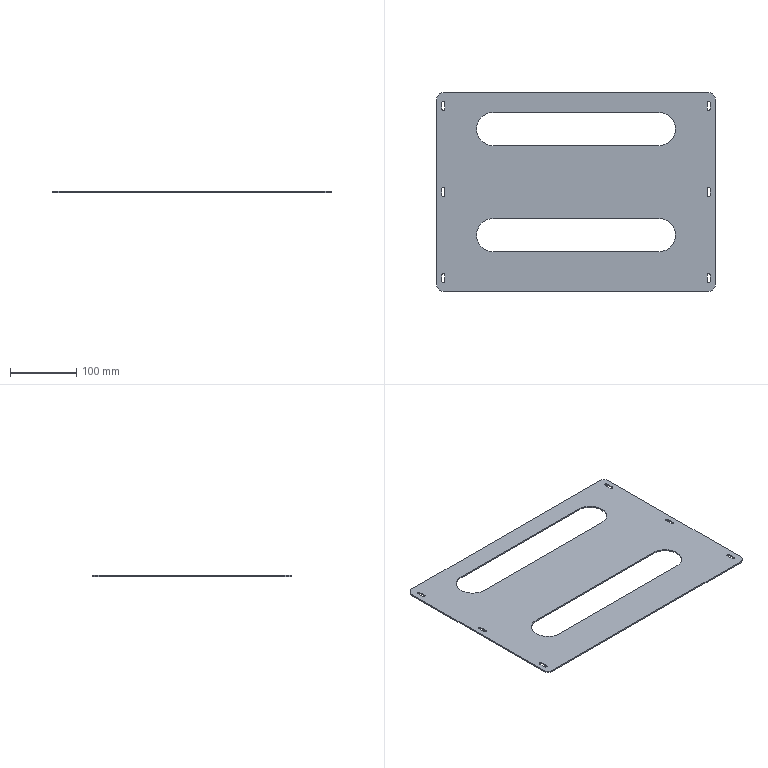Part | SolidWorks | features ICE 2, Extrusion 1, Fillet 1, HoleWzd 1, MirrorPattern 1 | 1 solid | 44 faces | box 420 x 300 x 2 mm | volume 193243 mm3 | cylinder 22 | plane 22 | commonest cylinder face diameters 4.5 x12 50 x6 20 x4
STEP:
#1=CARTESIAN_POINT('',(150.,-65.,0.));
#2=VERTEX_POINT('',#1);
#3=CARTESIAN_POINT('',(125.,-40.,0.));
#4=VERTEX_POINT('',#3);
#5=CARTESIAN_POINT('',(125.,-65.,0.));
#6=DIRECTION('',(0.,0.,1.));
#7=DIRECTION('',(1.,0.,0.));
#8=AXIS2_PLACEMENT_3D('',#5,#6,#7);
#9=CIRCLE('',#8,25.);
#10=EDGE_CURVE('',#2,#4,#9,.T.);
#11=ORIENTED_EDGE('',*,*,#10,.F.);
#12=CARTESIAN_POINT('',(150.,-65.,2.));
#13=VERTEX_POINT('',#12);
#14=CARTESIAN_POINT('',(150.,-65.,-8.));
#15=DIRECTION('',(0.,0.,1.));
#16=VECTOR('',#15,1000.);
#17=LINE('',#14,#16);
#18=EDGE_CURVE('',#2,#13,#17,.T.);
#19=ORIENTED_EDGE('',*,*,#18,.T.);
#20=CARTESIAN_POINT('',(125.,-40.,2.));
#21=VERTEX_POINT('',#20);
#22=CARTESIAN_POINT('',(125.,-65.,2.));
#23=DIRECTION('',(0.,0.,1.));
#24=DIRECTION('',(1.,0.,0.));
#25=AXIS2_PLACEMENT_3D('',#22,#23,#24);
#26=CIRCLE('',#25,25.);
#27=EDGE_CURVE('',#13,#21,#26,.T.);
#28=ORIENTED_EDGE('',*,*,#27,.T.);
#29=CARTESIAN_POINT('',(125.,-40.,-8.));
#30=DIRECTION('',(0.,0.,1.));
#31=VECTOR('',#30,1000.);
#32=LINE('',#29,#31);
#33=EDGE_CURVE('',#4,#21,#32,.T.);
#34=ORIENTED_EDGE('',*,*,#33,.F.);
#35=EDGE_LOOP('',(#11,#19,#28,#34));
#36=FACE_OUTER_BOUND('',#35,.T.);
#37=CARTESIAN_POINT('',(125.,-65.,-8.));
#38=DIRECTION('',(0.,0.,1.));
#39=DIRECTION('',(1.,0.,0.));
#40=AXIS2_PLACEMENT_3D('',#37,#38,#39);
#41=CYLINDRICAL_SURFACE('',#40,25.);
#42=ADVANCED_FACE('',(#36),#41,.F.);
#43=CARTESIAN_POINT('',(150.,95.,0.));
#44=VERTEX_POINT('',#43);
#45=CARTESIAN_POINT('',(125.,120.,0.));
#46=VERTEX_POINT('',#45);
#47=CARTESIAN_POINT('',(125.,95.,0.));
#48=DIRECTION('',(0.,0.,1.));
#49=DIRECTION('',(1.,0.,0.));
#50=AXIS2_PLACEMENT_3D('',#47,#48,#49);
#51=CIRCLE('',#50,25.);
#52=EDGE_CURVE('',#44,#46,#51,.T.);
#53=ORIENTED_EDGE('',*,*,#52,.F.);
#54=CARTESIAN_POINT('',(150.,95.,2.));
#55=VERTEX_POINT('',#54);
#56=CARTESIAN_POINT('',(150.,95.,-8.));
#57=DIRECTION('',(0.,0.,1.));
#58=VECTOR('',#57,1000.);
#59=LINE('',#56,#58);
#60=EDGE_CURVE('',#44,#55,#59,.T.);
#61=ORIENTED_EDGE('',*,*,#60,.T.);
#62=CARTESIAN_POINT('',(125.,120.,2.));
#63=VERTEX_POINT('',#62);
#64=CARTESIAN_POINT('',(125.,95.,2.));
#65=DIRECTION('',(0.,0.,1.));
#66=DIRECTION('',(1.,0.,0.));
#67=AXIS2_PLACEMENT_3D('',#64,#65,#66);
#68=CIRCLE('',#67,25.);
#69=EDGE_CURVE('',#55,#63,#68,.T.);
#70=ORIENTED_EDGE('',*,*,#69,.T.);
#71=CARTESIAN_POINT('',(125.,120.,-8.));
#72=DIRECTION('',(0.,0.,1.));
#73=VECTOR('',#72,1000.);
#74=LINE('',#71,#73);
#75=EDGE_CURVE('',#46,#63,#74,.T.);
#76=ORIENTED_EDGE('',*,*,#75,.F.);
#77=EDGE_LOOP('',(#53,#61,#70,#76));
#78=FACE_OUTER_BOUND('',#77,.T.);
#79=CARTESIAN_POINT('',(125.,95.,-8.));
#80=DIRECTION('',(0.,0.,1.));
#81=DIRECTION('',(1.,0.,0.));
#82=AXIS2_PLACEMENT_3D('',#79,#80,#81);
#83=CYLINDRICAL_SURFACE('',#82,25.);
#84=ADVANCED_FACE('',(#78),#83,.F.);
#85=CARTESIAN_POINT('',(210.,-140.,2.));
#86=VERTEX_POINT('',#85);
#87=CARTESIAN_POINT('',(210.,140.,2.));
#88=VERTEX_POINT('',#87);
#89=CARTESIAN_POINT('',(210.,150.,2.));
#90=DIRECTION('',(0.,1.,0.));
#91=VECTOR('',#90,1000.);
#92=LINE('',#89,#91);
#93=EDGE_CURVE('',#86,#88,#92,.T.);
#94=ORIENTED_EDGE('',*,*,#93,.F.);
#95=CARTESIAN_POINT('',(210.,-140.,0.));
#96=VERTEX_POINT('',#95);
#97=CARTESIAN_POINT('',(210.,-140.,2.));
#98=DIRECTION('',(0.,0.,-1.));
#99=VECTOR('',#98,1000.);
#100=LINE('',#97,#99);
#101=EDGE_CURVE('',#86,#96,#100,.T.);
#102=ORIENTED_EDGE('',*,*,#101,.T.);
#103=CARTESIAN_POINT('',(210.,140.,0.));
#104=VERTEX_POINT('',#103);
#105=CARTESIAN_POINT('',(210.,150.,0.));
#106=DIRECTION('',(0.,1.,0.));
#107=VECTOR('',#106,1000.);
#108=LINE('',#105,#107);
#109=EDGE_CURVE('',#96,#104,#108,.T.);
#110=ORIENTED_EDGE('',*,*,#109,.T.);
#111=CARTESIAN_POINT('',(210.,140.,2.));
#112=DIRECTION('',(0.,0.,1.));
#113=VECTOR('',#112,1000.);
#114=LINE('',#111,#113);
#115=EDGE_CURVE('',#104,#88,#114,.T.);
#116=ORIENTED_EDGE('',*,*,#115,.T.);
#117=EDGE_LOOP('',(#94,#102,#110,#116));
#118=FACE_OUTER_BOUND('',#117,.T.);
#119=CARTESIAN_POINT('',(210.,150.,2.));
#120=DIRECTION('',(-1.,0.,0.));
#121=DIRECTION('',(0.,0.,1.));
#122=AXIS2_PLACEMENT_3D('',#119,#120,#121);
#123=PLANE('',#122);
#124=ADVANCED_FACE('',(#118),#123,.F.);
#125=CARTESIAN_POINT('',(200.,150.,0.));
#126=VERTEX_POINT('',#125);
#127=CARTESIAN_POINT('',(-200.,150.,0.));
#128=VERTEX_POINT('',#127);
#129=CARTESIAN_POINT('',(-210.,150.,0.));
#130=DIRECTION('',(-1.,0.,0.));
#131=VECTOR('',#130,1000.);
#132=LINE('',#129,#131);
#133=EDGE_CURVE('',#126,#128,#132,.T.);
#134=ORIENTED_EDGE('',*,*,#133,.T.);
#135=CARTESIAN_POINT('',(-200.,150.,2.));
#136=VERTEX_POINT('',#135);
#137=CARTESIAN_POINT('',(-200.,150.,2.));
#138=DIRECTION('',(0.,0.,1.));
#139=VECTOR('',#138,1000.);
#140=LINE('',#137,#139);
#141=EDGE_CURVE('',#128,#136,#140,.T.);
#142=ORIENTED_EDGE('',*,*,#141,.T.);
#143=CARTESIAN_POINT('',(200.,150.,2.));
#144=VERTEX_POINT('',#143);
#145=CARTESIAN_POINT('',(-210.,150.,2.));
#146=DIRECTION('',(-1.,0.,0.));
#147=VECTOR('',#146,1000.);
#148=LINE('',#145,#147);
#149=EDGE_CURVE('',#144,#136,#148,.T.);
#150=ORIENTED_EDGE('',*,*,#149,.F.);
#151=CARTESIAN_POINT('',(200.,150.,2.));
#152=DIRECTION('',(0.,0.,-1.));
#153=VECTOR('',#152,1000.);
#154=LINE('',#151,#153);
#155=EDGE_CURVE('',#144,#126,#154,.T.);
#156=ORIENTED_EDGE('',*,*,#155,.T.);
#157=EDGE_LOOP('',(#134,#142,#150,#156));
#158=FACE_OUTER_BOUND('',#157,.T.);
#159=CARTESIAN_POINT('',(-210.,150.,2.));
#160=DIRECTION('',(0.,-1.,0.));
#161=DIRECTION('',(0.,0.,-1.));
#162=AXIS2_PLACEMENT_3D('',#159,#160,#161);
#163=PLANE('',#162);
#164=ADVANCED_FACE('',(#158),#163,.F.);
#165=CARTESIAN_POINT('',(-210.,140.,0.));
#166=VERTEX_POINT('',#165);
#167=CARTESIAN_POINT('',(-210.,-140.,0.));
#168=VERTEX_POINT('',#167);
#169=CARTESIAN_POINT('',(-210.,150.,0.));
#170=DIRECTION('',(0.,-1.,0.));
#171=VECTOR('',#170,1000.);
#172=LINE('',#169,#171);
#173=EDGE_CURVE('',#166,#168,#172,.T.);
#174=ORIENTED_EDGE('',*,*,#173,.T.);
#175=CARTESIAN_POINT('',(-210.,-140.,2.));
#176=VERTEX_POINT('',#175);
#177=CARTESIAN_POINT('',(-210.,-140.,2.));
#178=DIRECTION('',(0.,0.,1.));
#179=VECTOR('',#178,1000.);
#180=LINE('',#177,#179);
#181=EDGE_CURVE('',#168,#176,#180,.T.);
#182=ORIENTED_EDGE('',*,*,#181,.T.);
#183=CARTESIAN_POINT('',(-210.,140.,2.));
#184=VERTEX_POINT('',#183);
#185=CARTESIAN_POINT('',(-210.,150.,2.));
#186=DIRECTION('',(0.,-1.,0.));
#187=VECTOR('',#186,1000.);
#188=LINE('',#185,#187);
#189=EDGE_CURVE('',#184,#176,#188,.T.);
#190=ORIENTED_EDGE('',*,*,#189,.F.);
#191=CARTESIAN_POINT('',(-210.,140.,2.));
#192=DIRECTION('',(0.,0.,-1.));
#193=VECTOR('',#192,1000.);
#194=LINE('',#191,#193);
#195=EDGE_CURVE('',#184,#166,#194,.T.);
#196=ORIENTED_EDGE('',*,*,#195,.T.);
#197=EDGE_LOOP('',(#174,#182,#190,#196));
#198=FACE_OUTER_BOUND('',#197,.T.);
#199=CARTESIAN_POINT('',(-210.,150.,2.));
#200=DIRECTION('',(1.,0.,0.));
#201=DIRECTION('',(0.,0.,-1.));
#202=AXIS2_PLACEMENT_3D('',#199,#200,#201);
#203=PLANE('',#202);
#204=ADVANCED_FACE('',(#198),#203,.F.);
#205=CARTESIAN_POINT('',(-200.,-150.,2.));
#206=VERTEX_POINT('',#205);
#207=CARTESIAN_POINT('',(200.,-150.,2.));
#208=VERTEX_POINT('',#207);
#209=CARTESIAN_POINT('',(-210.,-150.,2.));
#210=DIRECTION('',(1.,0.,0.));
#211=VECTOR('',#210,1000.);
#212=LINE('',#209,#211);
#213=EDGE_CURVE('',#206,#208,#212,.T.);
#214=ORIENTED_EDGE('',*,*,#213,.F.);
#215=CARTESIAN_POINT('',(-200.,-150.,0.));
#216=VERTEX_POINT('',#215);
#217=CARTESIAN_POINT('',(-200.,-150.,2.));
#218=DIRECTION('',(0.,0.,-1.));
#219=VECTOR('',#218,1000.);
#220=LINE('',#217,#219);
#221=EDGE_CURVE('',#206,#216,#220,.T.);
#222=ORIENTED_EDGE('',*,*,#221,.T.);
#223=CARTESIAN_POINT('',(200.,-150.,0.));
#224=VERTEX_POINT('',#223);
#225=CARTESIAN_POINT('',(-210.,-150.,0.));
#226=DIRECTION('',(1.,0.,0.));
#227=VECTOR('',#226,1000.);
#228=LINE('',#225,#227);
#229=EDGE_CURVE('',#216,#224,#228,.T.);
#230=ORIENTED_EDGE('',*,*,#229,.T.);
#231=CARTESIAN_POINT('',(200.,-150.,2.));
#232=DIRECTION('',(0.,0.,1.));
#233=VECTOR('',#232,1000.);
#234=LINE('',#231,#233);
#235=EDGE_CURVE('',#224,#208,#234,.T.);
#236=ORIENTED_EDGE('',*,*,#235,.T.);
#237=EDGE_LOOP('',(#214,#222,#230,#236));
#238=FACE_OUTER_BOUND('',#237,.T.);
#239=CARTESIAN_POINT('',(-210.,-150.,2.));
#240=DIRECTION('',(0.,1.,0.));
#241=DIRECTION('',(0.,0.,1.));
#242=AXIS2_PLACEMENT_3D('',#239,#240,#241);
#243=PLANE('',#242);
#244=ADVANCED_FACE('',(#238),#243,.F.);
#245=CARTESIAN_POINT('',(-125.,-40.,2.));
#246=VERTEX_POINT('',#245);
#247=CARTESIAN_POINT('',(-125.,-90.,2.));
#248=VERTEX_POINT('',#247);
#249=CARTESIAN_POINT('',(-125.,-65.,2.));
#250=DIRECTION('',(0.,0.,1.));
#251=DIRECTION('',(1.,0.,0.));
#252=AXIS2_PLACEMENT_3D('',#249,#250,#251);
#253=CIRCLE('',#252,25.);
#254=EDGE_CURVE('',#246,#248,#253,.T.);
#255=ORIENTED_EDGE('',*,*,#254,.F.);
#256=CARTESIAN_POINT('',(-125.,-40.,2.));
#257=DIRECTION('',(-1.,0.,0.));
#258=VECTOR('',#257,1000.);
#259=LINE('',#256,#258);
#260=EDGE_CURVE('',#21,#246,#259,.T.);
#261=ORIENTED_EDGE('',*,*,#260,.F.);
#262=ORIENTED_EDGE('',*,*,#27,.F.);
#263=CARTESIAN_POINT('',(125.,-90.,2.));
#264=VERTEX_POINT('',#263);
#265=CARTESIAN_POINT('',(125.,-65.,2.));
#266=DIRECTION('',(0.,0.,1.));
#267=DIRECTION('',(1.,0.,0.));
#268=AXIS2_PLACEMENT_3D('',#265,#266,#267);
#269=CIRCLE('',#268,25.);
#270=EDGE_CURVE('',#264,#13,#269,.T.);
#271=ORIENTED_EDGE('',*,*,#270,.F.);
#272=CARTESIAN_POINT('',(-125.,-90.,2.));
#273=DIRECTION('',(1.,0.,0.));
#274=VECTOR('',#273,1000.);
#275=LINE('',#272,#274);
#276=EDGE_CURVE('',#248,#264,#275,.T.);
#277=ORIENTED_EDGE('',*,*,#276,.F.);
#278=EDGE_LOOP('',(#255,#261,#262,#271,#277));
#279=FACE_BOUND('',#278,.T.);
#280=CARTESIAN_POINT('',(125.,70.,2.));
#281=VERTEX_POINT('',#280);
#282=CARTESIAN_POINT('',(125.,95.,2.));
#283=DIRECTION('',(0.,0.,1.));
#284=DIRECTION('',(1.,0.,0.));
#285=AXIS2_PLACEMENT_3D('',#282,#283,#284);
#286=CIRCLE('',#285,25.);
#287=EDGE_CURVE('',#281,#55,#286,.T.);
#288=ORIENTED_EDGE('',*,*,#287,.F.);
#289=CARTESIAN_POINT('',(-125.,70.,2.));
#290=VERTEX_POINT('',#289);
#291=CARTESIAN_POINT('',(125.,70.,2.));
#292=DIRECTION('',(1.,0.,0.));
#293=VECTOR('',#292,1000.);
#294=LINE('',#291,#293);
#295=EDGE_CURVE('',#290,#281,#294,.T.);
#296=ORIENTED_EDGE('',*,*,#295,.F.);
#297=CARTESIAN_POINT('',(-125.,120.,2.));
#298=VERTEX_POINT('',#297);
#299=CARTESIAN_POINT('',(-125.,95.,2.));
#300=DIRECTION('',(0.,0.,1.));
#301=DIRECTION('',(1.,0.,0.));
#302=AXIS2_PLACEMENT_3D('',#299,#300,#301);
#303=CIRCLE('',#302,25.);
#304=EDGE_CURVE('',#298,#290,#303,.T.);
#305=ORIENTED_EDGE('',*,*,#304,.F.);
#306=CARTESIAN_POINT('',(125.,120.,2.));
#307=DIRECTION('',(-1.,0.,0.));
#308=VECTOR('',#307,1000.);
#309=LINE('',#306,#308);
#310=EDGE_CURVE('',#63,#298,#309,.T.);
#311=ORIENTED_EDGE('',*,*,#310,.F.);
#312=ORIENTED_EDGE('',*,*,#69,.F.);
#313=EDGE_LOOP('',(#288,#296,#305,#311,#312));
#314=FACE_BOUND('',#313,.T.);
#315=CARTESIAN_POINT('',(-202.25,-135.,2.));
#316=VERTEX_POINT('',#315);
#317=CARTESIAN_POINT('',(-197.75,-135.,2.));
#318=VERTEX_POINT('',#317);
#319=CARTESIAN_POINT('',(-200.,-135.,2.));
#320=DIRECTION('',(0.,0.,1.));
#321=DIRECTION('',(-1.,0.,0.));
#322=AXIS2_PLACEMENT_3D('',#319,#320,#321);
#323=CIRCLE('',#322,2.25);
#324=EDGE_CURVE('',#316,#318,#323,.T.);
#325=ORIENTED_EDGE('',*,*,#324,.F.);
#326=CARTESIAN_POINT('',(-202.25,-125.,2.));
#327=VERTEX_POINT('',#326);
#328=CARTESIAN_POINT('',(-202.25,-135.,2.));
#329=DIRECTION('',(0.,-1.,0.));
#330=VECTOR('',#329,1000.);
#331=LINE('',#328,#330);
#332=EDGE_CURVE('',#327,#316,#331,.T.);
#333=ORIENTED_EDGE('',*,*,#332,.F.);
#334=CARTESIAN_POINT('',(-197.75,-125.,2.));
#335=VERTEX_POINT('',#334);
#336=CARTESIAN_POINT('',(-200.,-125.,2.));
#337=DIRECTION('',(0.,0.,1.));
#338=DIRECTION('',(-1.,0.,0.));
#339=AXIS2_PLACEMENT_3D('',#336,#337,#338);
#340=CIRCLE('',#339,2.25);
#341=EDGE_CURVE('',#335,#327,#340,.T.);
#342=ORIENTED_EDGE('',*,*,#341,.F.);
#343=CARTESIAN_POINT('',(-197.75,-135.,2.));
#344=DIRECTION('',(0.,1.,0.));
#345=VECTOR('',#344,1000.);
#346=LINE('',#343,#345);
#347=EDGE_CURVE('',#318,#335,#346,.T.);
#348=ORIENTED_EDGE('',*,*,#347,.F.);
#349=EDGE_LOOP('',(#325,#333,#342,#348));
#350=FACE_BOUND('',#349,.T.);
#351=CARTESIAN_POINT('',(197.75,-5.,2.));
#352=VERTEX_POINT('',#351);
#353=CARTESIAN_POINT('',(202.25,-5.,2.));
#354=VERTEX_POINT('',#353);
#355=CARTESIAN_POINT('',(200.,-5.,2.));
#356=DIRECTION('',(0.,0.,1.));
#357=DIRECTION('',(-1.,0.,0.));
#358=AXIS2_PLACEMENT_3D('',#355,#356,#357);
#359=CIRCLE('',#358,2.25);
#360=EDGE_CURVE('',#352,#354,#359,.T.);
#361=ORIENTED_EDGE('',*,*,#360,.F.);
#362=CARTESIAN_POINT('',(197.75,5.,2.));
#363=VERTEX_POINT('',#362);
#364=CARTESIAN_POINT('',(197.75,-5.,2.));
#365=DIRECTION('',(0.,-1.,0.));
#366=VECTOR('',#365,1000.);
#367=LINE('',#364,#366);
#368=EDGE_CURVE('',#363,#352,#367,.T.);
#369=ORIENTED_EDGE('',*,*,#368,.F.);
#370=CARTESIAN_POINT('',(202.25,5.,2.));
#371=VERTEX_POINT('',#370);
#372=CARTESIAN_POINT('',(200.,5.,2.));
#373=DIRECTION('',(0.,0.,1.));
#374=DIRECTION('',(-1.,0.,0.));
#375=AXIS2_PLACEMENT_3D('',#372,#373,#374);
#376=CIRCLE('',#375,2.25);
#377=EDGE_CURVE('',#371,#363,#376,.T.);
#378=ORIENTED_EDGE('',*,*,#377,.F.);
#379=CARTESIAN_POINT('',(202.25,-5.,2.));
#380=DIRECTION('',(0.,1.,0.));
#381=VECTOR('',#380,1000.);
#382=LINE('',#379,#381);
#383=EDGE_CURVE('',#354,#371,#382,.T.);
#384=ORIENTED_EDGE('',*,*,#383,.F.);
#385=EDGE_LOOP('',(#361,#369,#378,#384));
#386=FACE_BOUND('',#385,.T.);
#387=CARTESIAN_POINT('',(202.25,135.,2.));
#388=VERTEX_POINT('',#387);
#389=CARTESIAN_POINT('',(197.75,135.,2.));
#390=VERTEX_POINT('',#389);
#391=CARTESIAN_POINT('',(200.,135.,2.));
#392=DIRECTION('',(0.,0.,1.));
#393=DIRECTION('',(-1.,0.,0.));
#394=AXIS2_PLACEMENT_3D('',#391,#392,#393);
#395=CIRCLE('',#394,2.25);
#396=EDGE_CURVE('',#388,#390,#395,.T.);
#397=ORIENTED_EDGE('',*,*,#396,.F.);
#398=CARTESIAN_POINT('',(202.25,125.,2.));
#399=VERTEX_POINT('',#398);
#400=CARTESIAN_POINT('',(202.25,135.,2.));
#401=DIRECTION('',(0.,1.,0.));
#402=VECTOR('',#401,1000.);
#403=LINE('',#400,#402);
#404=EDGE_CURVE('',#399,#388,#403,.T.);
#405=ORIENTED_EDGE('',*,*,#404,.F.);
#406=CARTESIAN_POINT('',(197.75,125.,2.));
#407=VERTEX_POINT('',#406);
#408=CARTESIAN_POINT('',(200.,125.,2.));
#409=DIRECTION('',(0.,0.,1.));
#410=DIRECTION('',(-1.,0.,0.));
#411=AXIS2_PLACEMENT_3D('',#408,#409,#410);
#412=CIRCLE('',#411,2.25);
#413=EDGE_CURVE('',#407,#399,#412,.T.);
#414=ORIENTED_EDGE('',*,*,#413,.F.);
#415=CARTESIAN_POINT('',(197.75,135.,2.));
#416=DIRECTION('',(0.,-1.,0.));
#417=VECTOR('',#416,1000.);
#418=LINE('',#415,#417);
#419=EDGE_CURVE('',#390,#407,#418,.T.);
#420=ORIENTED_EDGE('',*,*,#419,.F.);
#421=EDGE_LOOP('',(#397,#405,#414,#420));
#422=FACE_BOUND('',#421,.T.);
#423=CARTESIAN_POINT('',(-197.75,135.,2.));
#424=VERTEX_POINT('',#423);
#425=CARTESIAN_POINT('',(-202.25,135.,2.));
#426=VERTEX_POINT('',#425);
#427=CARTESIAN_POINT('',(-200.,135.,2.));
#428=DIRECTION('',(0.,0.,1.));
#429=DIRECTION('',(1.,0.,0.));
#430=AXIS2_PLACEMENT_3D('',#427,#428,#429);
#431=CIRCLE('',#430,2.25);
#432=EDGE_CURVE('',#424,#426,#431,.T.);
#433=ORIENTED_EDGE('',*,*,#432,.F.);
#434=CARTESIAN_POINT('',(-197.75,125.,2.));
#435=VERTEX_POINT('',#434);
#436=CARTESIAN_POINT('',(-197.75,135.,2.));
#437=DIRECTION('',(0.,1.,0.));
#438=VECTOR('',#437,1000.);
#439=LINE('',#436,#438);
#440=EDGE_CURVE('',#435,#424,#439,.T.);
#441=ORIENTED_EDGE('',*,*,#440,.F.);
#442=CARTESIAN_POINT('',(-202.25,125.,2.));
#443=VERTEX_POINT('',#442);
#444=CARTESIAN_POINT('',(-200.,125.,2.));
#445=DIRECTION('',(0.,0.,1.));
#446=DIRECTION('',(1.,0.,0.));
#447=AXIS2_PLACEMENT_3D('',#444,#445,#446);
#448=CIRCLE('',#447,2.25);
#449=EDGE_CURVE('',#443,#435,#448,.T.);
#450=ORIENTED_EDGE('',*,*,#449,.F.);
#451=CARTESIAN_POINT('',(-202.25,135.,2.));
#452=DIRECTION('',(0.,-1.,0.));
#453=VECTOR('',#452,1000.);
#454=LINE('',#451,#453);
#455=EDGE_CURVE('',#426,#443,#454,.T.);
#456=ORIENTED_EDGE('',*,*,#455,.F.);
#457=EDGE_LOOP('',(#433,#441,#450,#456));
#458=FACE_BOUND('',#457,.T.);
#459=CARTESIAN_POINT('',(-202.25,-5.,2.));
#460=VERTEX_POINT('',#459);
#461=CARTESIAN_POINT('',(-197.75,-5.,2.));
#462=VERTEX_POINT('',#461);
#463=CARTESIAN_POINT('',(-200.,-5.,2.));
#464=DIRECTION('',(0.,0.,1.));
#465=DIRECTION('',(1.,0.,0.));
#466=AXIS2_PLACEMENT_3D('',#463,#464,#465);
#467=CIRCLE('',#466,2.25);
#468=EDGE_CURVE('',#460,#462,#467,.T.);
#469=ORIENTED_EDGE('',*,*,#468,.F.);
#470=CARTESIAN_POINT('',(-202.25,5.,2.));
#471=VERTEX_POINT('',#470);
#472=CARTESIAN_POINT('',(-202.25,-5.,2.));
#473=DIRECTION('',(0.,-1.,0.));
#474=VECTOR('',#473,1000.);
#475=LINE('',#472,#474);
#476=EDGE_CURVE('',#471,#460,#475,.T.);
#477=ORIENTED_EDGE('',*,*,#476,.F.);
#478=CARTESIAN_POINT('',(-197.75,5.,2.));
#479=VERTEX_POINT('',#478);
#480=CARTESIAN_POINT('',(-200.,5.,2.));
#481=DIRECTION('',(0.,0.,1.));
#482=DIRECTION('',(1.,0.,0.));
#483=AXIS2_PLACEMENT_3D('',#480,#481,#482);
#484=CIRCLE('',#483,2.25);
#485=EDGE_CURVE('',#479,#471,#484,.T.);
#486=ORIENTED_EDGE('',*,*,#485,.F.);
#487=CARTESIAN_POINT('',(-197.75,-5.,2.));
#488=DIRECTION('',(0.,1.,0.));
#489=VECTOR('',#488,1000.);
#490=LINE('',#487,#489);
#491=EDGE_CURVE('',#462,#479,#490,.T.);
#492=ORIENTED_EDGE('',*,*,#491,.F.);
#493=EDGE_LOOP('',(#469,#477,#486,#492));
#494=FACE_BOUND('',#493,.T.);
#495=CARTESIAN_POINT('',(197.75,-135.,2.));
#496=VERTEX_POINT('',#495);
#497=CARTESIAN_POINT('',(202.25,-135.,2.));
#498=VERTEX_POINT('',#497);
#499=CARTESIAN_POINT('',(200.,-135.,2.));
#500=DIRECTION('',(0.,0.,1.));
#501=DIRECTION('',(1.,0.,0.));
#502=AXIS2_PLACEMENT_3D('',#499,#500,#501);
#503=CIRCLE('',#502,2.25);
#504=EDGE_CURVE('',#496,#498,#503,.T.);
#505=ORIENTED_EDGE('',*,*,#504,.F.);
#506=CARTESIAN_POINT('',(197.75,-125.,2.));
#507=VERTEX_POINT('',#506);
#508=CARTESIAN_POINT('',(197.75,-135.,2.));
#509=DIRECTION('',(0.,-1.,0.));
#510=VECTOR('',#509,1000.);
#511=LINE('',#508,#510);
#512=EDGE_CURVE('',#507,#496,#511,.T.);
#513=ORIENTED_EDGE('',*,*,#512,.F.);
#514=CARTESIAN_POINT('',(202.25,-125.,2.));
#515=VERTEX_POINT('',#514);
#516=CARTESIAN_POINT('',(200.,-125.,2.));
#517=DIRECTION('',(0.,0.,1.));
#518=DIRECTION('',(1.,0.,0.));
#519=AXIS2_PLACEMENT_3D('',#516,#517,#518);
#520=CIRCLE('',#519,2.25);
#521=EDGE_CURVE('',#515,#507,#520,.T.);
#522=ORIENTED_EDGE('',*,*,#521,.F.);
#523=CARTESIAN_POINT('',(202.25,-135.,2.));
#524=DIRECTION('',(0.,1.,0.));
#525=VECTOR('',#524,1000.);
#526=LINE('',#523,#525);
#527=EDGE_CURVE('',#498,#515,#526,.T.);
#528=ORIENTED_EDGE('',*,*,#527,.F.);
#529=EDGE_LOOP('',(#505,#513,#522,#528));
#530=FACE_BOUND('',#529,.T.);
#531=ORIENTED_EDGE('',*,*,#189,.T.);
#532=CARTESIAN_POINT('',(-200.,-140.,2.));
#533=DIRECTION('',(0.,0.,1.));
#534=DIRECTION('',(1.,0.,0.));
#535=AXIS2_PLACEMENT_3D('',#532,#533,#534);
#536=CIRCLE('',#535,10.);
#537=EDGE_CURVE('',#176,#206,#536,.T.);
#538=ORIENTED_EDGE('',*,*,#537,.T.);
#539=ORIENTED_EDGE('',*,*,#213,.T.);
#540=CARTESIAN_POINT('',(200.,-140.,2.));
#541=DIRECTION('',(0.,0.,1.));
#542=DIRECTION('',(1.,0.,0.));
#543=AXIS2_PLACEMENT_3D('',#540,#541,#542);
#544=CIRCLE('',#543,10.);
#545=EDGE_CURVE('',#208,#86,#544,.T.);
#546=ORIENTED_EDGE('',*,*,#545,.T.);
#547=ORIENTED_EDGE('',*,*,#93,.T.);
#548=CARTESIAN_POINT('',(200.,140.,2.));
#549=DIRECTION('',(0.,0.,1.));
#550=DIRECTION('',(1.,0.,0.));
#551=AXIS2_PLACEMENT_3D('',#548,#549,#550);
#552=CIRCLE('',#551,10.);
#553=EDGE_CURVE('',#88,#144,#552,.T.);
#554=ORIENTED_EDGE('',*,*,#553,.T.);
#555=ORIENTED_EDGE('',*,*,#149,.T.);
#556=CARTESIAN_POINT('',(-200.,140.,2.));
#557=DIRECTION('',(0.,0.,1.));
#558=DIRECTION('',(1.,0.,0.));
#559=AXIS2_PLACEMENT_3D('',#556,#557,#558);
#560=CIRCLE('',#559,10.);
#561=EDGE_CURVE('',#136,#184,#560,.T.);
#562=ORIENTED_EDGE('',*,*,#561,.T.);
#563=EDGE_LOOP('',(#531,#538,#539,#546,#547,#554,#555,#562));
#564=FACE_OUTER_BOUND('',#563,.T.);
#565=CARTESIAN_POINT('',(0.,0.,2.));
#566=DIRECTION('',(0.,0.,1.));
#567=DIRECTION('',(1.,0.,0.));
#568=AXIS2_PLACEMENT_3D('',#565,#566,#567);
#569=PLANE('',#568);
#570=ADVANCED_FACE('',(#279,#314,#350,#386,#422,#458,#494,#530,#564),#569,.T.);
#571=CARTESIAN_POINT('',(-125.,-40.,0.));
#572=VERTEX_POINT('',#571);
#573=CARTESIAN_POINT('',(0.,-40.,0.));
#574=DIRECTION('',(-1.,0.,0.));
#575=VECTOR('',#574,1000.);
#576=LINE('',#573,#575);
#577=EDGE_CURVE('',#4,#572,#576,.T.);
#578=ORIENTED_EDGE('',*,*,#577,.T.);
#579=CARTESIAN_POINT('',(-125.,-90.,0.));
#580=VERTEX_POINT('',#579);
#581=CARTESIAN_POINT('',(-125.,-65.,0.));
#582=DIRECTION('',(0.,0.,1.));
#583=DIRECTION('',(1.,0.,0.));
#584=AXIS2_PLACEMENT_3D('',#581,#582,#583);
#585=CIRCLE('',#584,25.);
#586=EDGE_CURVE('',#572,#580,#585,.T.);
#587=ORIENTED_EDGE('',*,*,#586,.T.);
#588=CARTESIAN_POINT('',(125.,-90.,0.));
#589=VERTEX_POINT('',#588);
#590=CARTESIAN_POINT('',(0.,-90.,0.));
#591=DIRECTION('',(1.,0.,0.));
#592=VECTOR('',#591,1000.);
#593=LINE('',#590,#592);
#594=EDGE_CURVE('',#580,#589,#593,.T.);
#595=ORIENTED_EDGE('',*,*,#594,.T.);
#596=CARTESIAN_POINT('',(125.,-65.,0.));
#597=DIRECTION('',(0.,0.,1.));
#598=DIRECTION('',(1.,0.,0.));
#599=AXIS2_PLACEMENT_3D('',#596,#597,#598);
#600=CIRCLE('',#599,25.);
#601=EDGE_CURVE('',#589,#2,#600,.T.);
#602=ORIENTED_EDGE('',*,*,#601,.T.);
#603=ORIENTED_EDGE('',*,*,#10,.T.);
#604=EDGE_LOOP('',(#578,#587,#595,#602,#603));
#605=FACE_BOUND('',#604,.T.);
#606=CARTESIAN_POINT('',(-125.,70.,0.));
#607=VERTEX_POINT('',#606);
#608=CARTESIAN_POINT('',(125.,70.,0.));
#609=VERTEX_POINT('',#608);
#610=CARTESIAN_POINT('',(0.,70.,0.));
#611=DIRECTION('',(1.,0.,0.));
#612=VECTOR('',#611,1000.);
#613=LINE('',#610,#612);
#614=EDGE_CURVE('',#607,#609,#613,.T.);
#615=ORIENTED_EDGE('',*,*,#614,.T.);
#616=CARTESIAN_POINT('',(125.,95.,0.));
#617=DIRECTION('',(0.,0.,1.));
#618=DIRECTION('',(1.,0.,0.));
#619=AXIS2_PLACEMENT_3D('',#616,#617,#618);
#620=CIRCLE('',#619,25.);
#621=EDGE_CURVE('',#609,#44,#620,.T.);
#622=ORIENTED_EDGE('',*,*,#621,.T.);
#623=ORIENTED_EDGE('',*,*,#52,.T.);
#624=CARTESIAN_POINT('',(-125.,120.,0.));
#625=VERTEX_POINT('',#624);
#626=CARTESIAN_POINT('',(0.,120.,0.));
#627=DIRECTION('',(-1.,0.,0.));
#628=VECTOR('',#627,1000.);
#629=LINE('',#626,#628);
#630=EDGE_CURVE('',#46,#625,#629,.T.);
#631=ORIENTED_EDGE('',*,*,#630,.T.);
#632=CARTESIAN_POINT('',(-125.,95.,0.));
#633=DIRECTION('',(0.,0.,1.));
#634=DIRECTION('',(1.,0.,0.));
#635=AXIS2_PLACEMENT_3D('',#632,#633,#634);
#636=CIRCLE('',#635,25.);
#637=EDGE_CURVE('',#625,#607,#636,.T.);
#638=ORIENTED_EDGE('',*,*,#637,.T.);
#639=EDGE_LOOP('',(#615,#622,#623,#631,#638));
#640=FACE_BOUND('',#639,.T.);
#641=CARTESIAN_POINT('',(-202.25,-125.,0.));
#642=VERTEX_POINT('',#641);
#643=CARTESIAN_POINT('',(-202.25,-135.,0.));
#644=VERTEX_POINT('',#643);
#645=CARTESIAN_POINT('',(-202.25,0.,0.));
#646=DIRECTION('',(0.,-1.,0.));
#647=VECTOR('',#646,1000.);
#648=LINE('',#645,#647);
#649=EDGE_CURVE('',#642,#644,#648,.T.);
#650=ORIENTED_EDGE('',*,*,#649,.T.);
#651=CARTESIAN_POINT('',(-197.75,-135.,0.));
#652=VERTEX_POINT('',#651);
#653=CARTESIAN_POINT('',(-200.,-135.,0.));
#654=DIRECTION('',(0.,0.,1.));
#655=DIRECTION('',(1.,0.,0.));
#656=AXIS2_PLACEMENT_3D('',#653,#654,#655);
#657=CIRCLE('',#656,2.25);
#658=EDGE_CURVE('',#644,#652,#657,.T.);
#659=ORIENTED_EDGE('',*,*,#658,.T.);
#660=CARTESIAN_POINT('',(-197.75,-125.,0.));
#661=VERTEX_POINT('',#660);
#662=CARTESIAN_POINT('',(-197.75,0.,0.));
#663=DIRECTION('',(0.,1.,0.));
#664=VECTOR('',#663,1000.);
#665=LINE('',#662,#664);
#666=EDGE_CURVE('',#652,#661,#665,.T.);
#667=ORIENTED_EDGE('',*,*,#666,.T.);
#668=CARTESIAN_POINT('',(-200.,-125.,0.));
#669=DIRECTION('',(0.,0.,1.));
#670=DIRECTION('',(1.,0.,0.));
#671=AXIS2_PLACEMENT_3D('',#668,#669,#670);
#672=CIRCLE('',#671,2.25);
#673=EDGE_CURVE('',#661,#642,#672,.T.);
#674=ORIENTED_EDGE('',*,*,#673,.T.);
#675=EDGE_LOOP('',(#650,#659,#667,#674));
#676=FACE_BOUND('',#675,.T.);
#677=CARTESIAN_POINT('',(197.75,5.,0.));
#678=VERTEX_POINT('',#677);
#679=CARTESIAN_POINT('',(197.75,-5.,0.));
#680=VERTEX_POINT('',#679);
#681=CARTESIAN_POINT('',(197.75,0.,0.));
#682=DIRECTION('',(0.,-1.,0.));
#683=VECTOR('',#682,1000.);
#684=LINE('',#681,#683);
#685=EDGE_CURVE('',#678,#680,#684,.T.);
#686=ORIENTED_EDGE('',*,*,#685,.T.);
#687=CARTESIAN_POINT('',(202.25,-5.,0.));
#688=VERTEX_POINT('',#687);
#689=CARTESIAN_POINT('',(200.,-5.,0.));
#690=DIRECTION('',(0.,0.,1.));
#691=DIRECTION('',(1.,0.,0.));
#692=AXIS2_PLACEMENT_3D('',#689,#690,#691);
#693=CIRCLE('',#692,2.25);
#694=EDGE_CURVE('',#680,#688,#693,.T.);
#695=ORIENTED_EDGE('',*,*,#694,.T.);
#696=CARTESIAN_POINT('',(202.25,5.,0.));
#697=VERTEX_POINT('',#696);
#698=CARTESIAN_POINT('',(202.25,0.,0.));
#699=DIRECTION('',(0.,1.,0.));
#700=VECTOR('',#699,1000.);
#701=LINE('',#698,#700);
#702=EDGE_CURVE('',#688,#697,#701,.T.);
#703=ORIENTED_EDGE('',*,*,#702,.T.);
#704=CARTESIAN_POINT('',(200.,5.,0.));
#705=DIRECTION('',(0.,0.,1.));
#706=DIRECTION('',(1.,0.,0.));
#707=AXIS2_PLACEMENT_3D('',#704,#705,#706);
#708=CIRCLE('',#707,2.25);
#709=EDGE_CURVE('',#697,#678,#708,.T.);
#710=ORIENTED_EDGE('',*,*,#709,.T.);
#711=EDGE_LOOP('',(#686,#695,#703,#710));
#712=FACE_BOUND('',#711,.T.);
#713=CARTESIAN_POINT('',(202.25,125.,0.));
#714=VERTEX_POINT('',#713);
#715=CARTESIAN_POINT('',(202.25,135.,0.));
#716=VERTEX_POINT('',#715);
#717=CARTESIAN_POINT('',(202.25,0.,0.));
#718=DIRECTION('',(0.,1.,0.));
#719=VECTOR('',#718,1000.);
#720=LINE('',#717,#719);
#721=EDGE_CURVE('',#714,#716,#720,.T.);
#722=ORIENTED_EDGE('',*,*,#721,.T.);
#723=CARTESIAN_POINT('',(197.75,135.,0.));
#724=VERTEX_POINT('',#723);
#725=CARTESIAN_POINT('',(200.,135.,0.));
#726=DIRECTION('',(0.,0.,1.));
#727=DIRECTION('',(1.,0.,0.));
#728=AXIS2_PLACEMENT_3D('',#725,#726,#727);
#729=CIRCLE('',#728,2.25);
#730=EDGE_CURVE('',#716,#724,#729,.T.);
#731=ORIENTED_EDGE('',*,*,#730,.T.);
#732=CARTESIAN_POINT('',(197.75,125.,0.));
#733=VERTEX_POINT('',#732);
#734=CARTESIAN_POINT('',(197.75,0.,0.));
#735=DIRECTION('',(0.,-1.,0.));
#736=VECTOR('',#735,1000.);
#737=LINE('',#734,#736);
#738=EDGE_CURVE('',#724,#733,#737,.T.);
#739=ORIENTED_EDGE('',*,*,#738,.T.);
#740=CARTESIAN_POINT('',(200.,125.,0.));
#741=DIRECTION('',(0.,0.,1.));
#742=DIRECTION('',(1.,0.,0.));
#743=AXIS2_PLACEMENT_3D('',#740,#741,#742);
#744=CIRCLE('',#743,2.25);
#745=EDGE_CURVE('',#733,#714,#744,.T.);
#746=ORIENTED_EDGE('',*,*,#745,.T.);
#747=EDGE_LOOP('',(#722,#731,#739,#746));
#748=FACE_BOUND('',#747,.T.);
#749=CARTESIAN_POINT('',(-197.75,125.,0.));
#750=VERTEX_POINT('',#749);
#751=CARTESIAN_POINT('',(-197.75,135.,0.));
#752=VERTEX_POINT('',#751);
#753=CARTESIAN_POINT('',(-197.75,0.,0.));
#754=DIRECTION('',(0.,1.,0.));
#755=VECTOR('',#754,1000.);
#756=LINE('',#753,#755);
#757=EDGE_CURVE('',#750,#752,#756,.T.);
#758=ORIENTED_EDGE('',*,*,#757,.T.);
#759=CARTESIAN_POINT('',(-202.25,135.,0.));
#760=VERTEX_POINT('',#759);
#761=CARTESIAN_POINT('',(-200.,135.,0.));
#762=DIRECTION('',(0.,0.,1.));
#763=DIRECTION('',(1.,0.,0.));
#764=AXIS2_PLACEMENT_3D('',#761,#762,#763);
#765=CIRCLE('',#764,2.25);
#766=EDGE_CURVE('',#752,#760,#765,.T.);
#767=ORIENTED_EDGE('',*,*,#766,.T.);
#768=CARTESIAN_POINT('',(-202.25,125.,0.));
#769=VERTEX_POINT('',#768);
#770=CARTESIAN_POINT('',(-202.25,0.,0.));
#771=DIRECTION('',(0.,-1.,0.));
#772=VECTOR('',#771,1000.);
#773=LINE('',#770,#772);
#774=EDGE_CURVE('',#760,#769,#773,.T.);
#775=ORIENTED_EDGE('',*,*,#774,.T.);
#776=CARTESIAN_POINT('',(-200.,125.,0.));
#777=DIRECTION('',(0.,0.,1.));
#778=DIRECTION('',(1.,0.,0.));
#779=AXIS2_PLACEMENT_3D('',#776,#777,#778);
#780=CIRCLE('',#779,2.25);
#781=EDGE_CURVE('',#769,#750,#780,.T.);
#782=ORIENTED_EDGE('',*,*,#781,.T.);
#783=EDGE_LOOP('',(#758,#767,#775,#782));
#784=FACE_BOUND('',#783,.T.);
#785=CARTESIAN_POINT('',(-202.25,5.,0.));
#786=VERTEX_POINT('',#785);
#787=CARTESIAN_POINT('',(-202.25,-5.,0.));
#788=VERTEX_POINT('',#787);
#789=CARTESIAN_POINT('',(-202.25,0.,0.));
#790=DIRECTION('',(0.,-1.,0.));
#791=VECTOR('',#790,1000.);
#792=LINE('',#789,#791);
#793=EDGE_CURVE('',#786,#788,#792,.T.);
#794=ORIENTED_EDGE('',*,*,#793,.T.);
#795=CARTESIAN_POINT('',(-197.75,-5.,0.));
#796=VERTEX_POINT('',#795);
#797=CARTESIAN_POINT('',(-200.,-5.,0.));
#798=DIRECTION('',(0.,0.,1.));
#799=DIRECTION('',(1.,0.,0.));
#800=AXIS2_PLACEMENT_3D('',#797,#798,#799);
#801=CIRCLE('',#800,2.25);
#802=EDGE_CURVE('',#788,#796,#801,.T.);
#803=ORIENTED_EDGE('',*,*,#802,.T.);
#804=CARTESIAN_POINT('',(-197.75,5.,0.));
#805=VERTEX_POINT('',#804);
#806=CARTESIAN_POINT('',(-197.75,0.,0.));
#807=DIRECTION('',(0.,1.,0.));
#808=VECTOR('',#807,1000.);
#809=LINE('',#806,#808);
#810=EDGE_CURVE('',#796,#805,#809,.T.);
#811=ORIENTED_EDGE('',*,*,#810,.T.);
#812=CARTESIAN_POINT('',(-200.,5.,0.));
#813=DIRECTION('',(0.,0.,1.));
#814=DIRECTION('',(1.,0.,0.));
#815=AXIS2_PLACEMENT_3D('',#812,#813,#814);
#816=CIRCLE('',#815,2.25);
#817=EDGE_CURVE('',#805,#786,#816,.T.);
#818=ORIENTED_EDGE('',*,*,#817,.T.);
#819=EDGE_LOOP('',(#794,#803,#811,#818));
#820=FACE_BOUND('',#819,.T.);
#821=CARTESIAN_POINT('',(197.75,-125.,0.));
#822=VERTEX_POINT('',#821);
#823=CARTESIAN_POINT('',(197.75,-135.,0.));
#824=VERTEX_POINT('',#823);
#825=CARTESIAN_POINT('',(197.75,0.,0.));
#826=DIRECTION('',(0.,-1.,0.));
#827=VECTOR('',#826,1000.);
#828=LINE('',#825,#827);
#829=EDGE_CURVE('',#822,#824,#828,.T.);
#830=ORIENTED_EDGE('',*,*,#829,.T.);
#831=CARTESIAN_POINT('',(202.25,-135.,0.));
#832=VERTEX_POINT('',#831);
#833=CARTESIAN_POINT('',(200.,-135.,0.));
#834=DIRECTION('',(0.,0.,1.));
#835=DIRECTION('',(1.,0.,0.));
#836=AXIS2_PLACEMENT_3D('',#833,#834,#835);
#837=CIRCLE('',#836,2.25);
#838=EDGE_CURVE('',#824,#832,#837,.T.);
#839=ORIENTED_EDGE('',*,*,#838,.T.);
#840=CARTESIAN_POINT('',(202.25,-125.,0.));
#841=VERTEX_POINT('',#840);
#842=CARTESIAN_POINT('',(202.25,0.,0.));
#843=DIRECTION('',(0.,1.,0.));
#844=VECTOR('',#843,1000.);
#845=LINE('',#842,#844);
#846=EDGE_CURVE('',#832,#841,#845,.T.);
#847=ORIENTED_EDGE('',*,*,#846,.T.);
#848=CARTESIAN_POINT('',(200.,-125.,0.));
#849=DIRECTION('',(0.,0.,1.));
#850=DIRECTION('',(1.,0.,0.));
#851=AXIS2_PLACEMENT_3D('',#848,#849,#850);
#852=CIRCLE('',#851,2.25);
#853=EDGE_CURVE('',#841,#822,#852,.T.);
#854=ORIENTED_EDGE('',*,*,#853,.T.);
#855=EDGE_LOOP('',(#830,#839,#847,#854));
#856=FACE_BOUND('',#855,.T.);
#857=ORIENTED_EDGE('',*,*,#229,.F.);
#858=CARTESIAN_POINT('',(-200.,-140.,0.));
#859=DIRECTION('',(0.,0.,-1.));
#860=DIRECTION('',(1.,0.,0.));
#861=AXIS2_PLACEMENT_3D('',#858,#859,#860);
#862=CIRCLE('',#861,10.);
#863=EDGE_CURVE('',#216,#168,#862,.T.);
#864=ORIENTED_EDGE('',*,*,#863,.T.);
#865=ORIENTED_EDGE('',*,*,#173,.F.);
#866=CARTESIAN_POINT('',(-200.,140.,0.));
#867=DIRECTION('',(0.,0.,-1.));
#868=DIRECTION('',(1.,0.,0.));
#869=AXIS2_PLACEMENT_3D('',#866,#867,#868);
#870=CIRCLE('',#869,10.);
#871=EDGE_CURVE('',#166,#128,#870,.T.);
#872=ORIENTED_EDGE('',*,*,#871,.T.);
#873=ORIENTED_EDGE('',*,*,#133,.F.);
#874=CARTESIAN_POINT('',(200.,140.,0.));
#875=DIRECTION('',(0.,0.,-1.));
#876=DIRECTION('',(1.,0.,0.));
#877=AXIS2_PLACEMENT_3D('',#874,#875,#876);
#878=CIRCLE('',#877,10.);
#879=EDGE_CURVE('',#126,#104,#878,.T.);
#880=ORIENTED_EDGE('',*,*,#879,.T.);
#881=ORIENTED_EDGE('',*,*,#109,.F.);
#882=CARTESIAN_POINT('',(200.,-140.,0.));
#883=DIRECTION('',(0.,0.,-1.));
#884=DIRECTION('',(1.,0.,0.));
#885=AXIS2_PLACEMENT_3D('',#882,#883,#884);
#886=CIRCLE('',#885,10.);
#887=EDGE_CURVE('',#96,#224,#886,.T.);
#888=ORIENTED_EDGE('',*,*,#887,.T.);
#889=EDGE_LOOP('',(#857,#864,#865,#872,#873,#880,#881,#888));
#890=FACE_OUTER_BOUND('',#889,.T.);
#891=CARTESIAN_POINT('',(0.,0.,0.));
#892=DIRECTION('',(0.,0.,1.));
#893=DIRECTION('',(1.,0.,0.));
#894=AXIS2_PLACEMENT_3D('',#891,#892,#893);
#895=PLANE('',#894);
#896=ADVANCED_FACE('',(#605,#640,#676,#712,#748,#784,#820,#856,#890),#895,.F.);
#897=CARTESIAN_POINT('',(197.75,-135.,-8.));
#898=DIRECTION('',(0.,0.,1.));
#899=VECTOR('',#898,1000.);
#900=LINE('',#897,#899);
#901=EDGE_CURVE('',#824,#496,#900,.T.);
#902=ORIENTED_EDGE('',*,*,#901,.T.);
#903=ORIENTED_EDGE('',*,*,#504,.T.);
#904=CARTESIAN_POINT('',(202.25,-135.,-8.));
#905=DIRECTION('',(0.,0.,1.));
#906=VECTOR('',#905,1000.);
#907=LINE('',#904,#906);
#908=EDGE_CURVE('',#832,#498,#907,.T.);
#909=ORIENTED_EDGE('',*,*,#908,.F.);
#910=ORIENTED_EDGE('',*,*,#838,.F.);
#911=EDGE_LOOP('',(#902,#903,#909,#910));
#912=FACE_OUTER_BOUND('',#911,.T.);
#913=CARTESIAN_POINT('',(200.,-135.,-8.));
#914=DIRECTION('',(0.,0.,1.));
#915=DIRECTION('',(1.,0.,0.));
#916=AXIS2_PLACEMENT_3D('',#913,#914,#915);
#917=CYLINDRICAL_SURFACE('',#916,2.25);
#918=ADVANCED_FACE('',(#912),#917,.F.);
#919=CARTESIAN_POINT('',(197.75,-125.,-8.));
#920=DIRECTION('',(0.,0.,1.));
#921=VECTOR('',#920,1000.);
#922=LINE('',#919,#921);
#923=EDGE_CURVE('',#822,#507,#922,.T.);
#924=ORIENTED_EDGE('',*,*,#923,.T.);
#925=ORIENTED_EDGE('',*,*,#512,.T.);
#926=ORIENTED_EDGE('',*,*,#901,.F.);
#927=ORIENTED_EDGE('',*,*,#829,.F.);
#928=EDGE_LOOP('',(#924,#925,#926,#927));
#929=FACE_OUTER_BOUND('',#928,.T.);
#930=CARTESIAN_POINT('',(197.75,-135.,-8.));
#931=DIRECTION('',(-1.,0.,0.));
#932=DIRECTION('',(0.,0.,1.));
#933=AXIS2_PLACEMENT_3D('',#930,#931,#932);
#934=PLANE('',#933);
#935=ADVANCED_FACE('',(#929),#934,.F.);
#936=CARTESIAN_POINT('',(202.25,-125.,-8.));
#937=DIRECTION('',(0.,0.,1.));
#938=VECTOR('',#937,1000.);
#939=LINE('',#936,#938);
#940=EDGE_CURVE('',#841,#515,#939,.T.);
#941=ORIENTED_EDGE('',*,*,#940,.T.);
#942=ORIENTED_EDGE('',*,*,#521,.T.);
#943=ORIENTED_EDGE('',*,*,#923,.F.);
#944=ORIENTED_EDGE('',*,*,#853,.F.);
#945=EDGE_LOOP('',(#941,#942,#943,#944));
#946=FACE_OUTER_BOUND('',#945,.T.);
#947=CARTESIAN_POINT('',(200.,-125.,-8.));
#948=DIRECTION('',(0.,0.,1.));
#949=DIRECTION('',(1.,0.,0.));
#950=AXIS2_PLACEMENT_3D('',#947,#948,#949);
#951=CYLINDRICAL_SURFACE('',#950,2.25);
#952=ADVANCED_FACE('',(#946),#951,.F.);
#953=ORIENTED_EDGE('',*,*,#908,.T.);
#954=ORIENTED_EDGE('',*,*,#527,.T.);
#955=ORIENTED_EDGE('',*,*,#940,.F.);
#956=ORIENTED_EDGE('',*,*,#846,.F.);
#957=EDGE_LOOP('',(#953,#954,#955,#956));
#958=FACE_OUTER_BOUND('',#957,.T.);
#959=CARTESIAN_POINT('',(202.25,-135.,-8.));
#960=DIRECTION('',(1.,0.,0.));
#961=DIRECTION('',(0.,0.,-1.));
#962=AXIS2_PLACEMENT_3D('',#959,#960,#961);
#963=PLANE('',#962);
#964=ADVANCED_FACE('',(#958),#963,.F.);
#965=CARTESIAN_POINT('',(-202.25,-5.,-8.));
#966=DIRECTION('',(0.,0.,1.));
#967=VECTOR('',#966,1000.);
#968=LINE('',#965,#967);
#969=EDGE_CURVE('',#788,#460,#968,.T.);
#970=ORIENTED_EDGE('',*,*,#969,.T.);
#971=ORIENTED_EDGE('',*,*,#468,.T.);
#972=CARTESIAN_POINT('',(-197.75,-5.,-8.));
#973=DIRECTION('',(0.,0.,1.));
#974=VECTOR('',#973,1000.);
#975=LINE('',#972,#974);
#976=EDGE_CURVE('',#796,#462,#975,.T.);
#977=ORIENTED_EDGE('',*,*,#976,.F.);
#978=ORIENTED_EDGE('',*,*,#802,.F.);
#979=EDGE_LOOP('',(#970,#971,#977,#978));
#980=FACE_OUTER_BOUND('',#979,.T.);
#981=CARTESIAN_POINT('',(-200.,-5.,-8.));
#982=DIRECTION('',(0.,0.,1.));
#983=DIRECTION('',(1.,0.,0.));
#984=AXIS2_PLACEMENT_3D('',#981,#982,#983);
#985=CYLINDRICAL_SURFACE('',#984,2.25);
#986=ADVANCED_FACE('',(#980),#985,.F.);
#987=CARTESIAN_POINT('',(-202.25,5.,-8.));
#988=DIRECTION('',(0.,0.,1.));
#989=VECTOR('',#988,1000.);
#990=LINE('',#987,#989);
#991=EDGE_CURVE('',#786,#471,#990,.T.);
#992=ORIENTED_EDGE('',*,*,#991,.T.);
#993=ORIENTED_EDGE('',*,*,#476,.T.);
#994=ORIENTED_EDGE('',*,*,#969,.F.);
#995=ORIENTED_EDGE('',*,*,#793,.F.);
#996=EDGE_LOOP('',(#992,#993,#994,#995));
#997=FACE_OUTER_BOUND('',#996,.T.);
#998=CARTESIAN_POINT('',(-202.25,-5.,-8.));
#999=DIRECTION('',(-1.,0.,0.));
#1000=DIRECTION('',(0.,0.,1.));
#1001=AXIS2_PLACEMENT_3D('',#998,#999,#1000);
#1002=PLANE('',#1001);
#1003=ADVANCED_FACE('',(#997),#1002,.F.);
#1004=CARTESIAN_POINT('',(-197.75,5.,-8.));
#1005=DIRECTION('',(0.,0.,1.));
#1006=VECTOR('',#1005,1000.);
#1007=LINE('',#1004,#1006);
#1008=EDGE_CURVE('',#805,#479,#1007,.T.);
#1009=ORIENTED_EDGE('',*,*,#1008,.T.);
#1010=ORIENTED_EDGE('',*,*,#485,.T.);
#1011=ORIENTED_EDGE('',*,*,#991,.F.);
#1012=ORIENTED_EDGE('',*,*,#817,.F.);
#1013=EDGE_LOOP('',(#1009,#1010,#1011,#1012));
#1014=FACE_OUTER_BOUND('',#1013,.T.);
#1015=CARTESIAN_POINT('',(-200.,5.,-8.));
#1016=DIRECTION('',(0.,0.,1.));
#1017=DIRECTION('',(1.,0.,0.));
#1018=AXIS2_PLACEMENT_3D('',#1015,#1016,#1017);
#1019=CYLINDRICAL_SURFACE('',#1018,2.25);
#1020=ADVANCED_FACE('',(#1014),#1019,.F.);
#1021=ORIENTED_EDGE('',*,*,#976,.T.);
#1022=ORIENTED_EDGE('',*,*,#491,.T.);
#1023=ORIENTED_EDGE('',*,*,#1008,.F.);
#1024=ORIENTED_EDGE('',*,*,#810,.F.);
#1025=EDGE_LOOP('',(#1021,#1022,#1023,#1024));
#1026=FACE_OUTER_BOUND('',#1025,.T.);
#1027=CARTESIAN_POINT('',(-197.75,-5.,-8.));
#1028=DIRECTION('',(1.,0.,0.));
#1029=DIRECTION('',(0.,0.,-1.));
#1030=AXIS2_PLACEMENT_3D('',#1027,#1028,#1029);
#1031=PLANE('',#1030);
#1032=ADVANCED_FACE('',(#1026),#1031,.F.);
#1033=CARTESIAN_POINT('',(-197.75,135.,-8.));
#1034=DIRECTION('',(0.,0.,1.));
#1035=VECTOR('',#1034,1000.);
#1036=LINE('',#1033,#1035);
#1037=EDGE_CURVE('',#752,#424,#1036,.T.);
#1038=ORIENTED_EDGE('',*,*,#1037,.T.);
#1039=ORIENTED_EDGE('',*,*,#432,.T.);
#1040=CARTESIAN_POINT('',(-202.25,135.,-8.));
#1041=DIRECTION('',(0.,0.,1.));
#1042=VECTOR('',#1041,1000.);
#1043=LINE('',#1040,#1042);
#1044=EDGE_CURVE('',#760,#426,#1043,.T.);
#1045=ORIENTED_EDGE('',*,*,#1044,.F.);
#1046=ORIENTED_EDGE('',*,*,#766,.F.);
#1047=EDGE_LOOP('',(#1038,#1039,#1045,#1046));
#1048=FACE_OUTER_BOUND('',#1047,.T.);
#1049=CARTESIAN_POINT('',(-200.,135.,-8.));
#1050=DIRECTION('',(0.,0.,1.));
#1051=DIRECTION('',(1.,0.,0.));
#1052=AXIS2_PLACEMENT_3D('',#1049,#1050,#1051);
#1053=CYLINDRICAL_SURFACE('',#1052,2.25);
#1054=ADVANCED_FACE('',(#1048),#1053,.F.);
#1055=CARTESIAN_POINT('',(-197.75,125.,-8.));
#1056=DIRECTION('',(0.,0.,1.));
#1057=VECTOR('',#1056,1000.);
#1058=LINE('',#1055,#1057);
#1059=EDGE_CURVE('',#750,#435,#1058,.T.);
#1060=ORIENTED_EDGE('',*,*,#1059,.T.);
#1061=ORIENTED_EDGE('',*,*,#440,.T.);
#1062=ORIENTED_EDGE('',*,*,#1037,.F.);
#1063=ORIENTED_EDGE('',*,*,#757,.F.);
#1064=EDGE_LOOP('',(#1060,#1061,#1062,#1063));
#1065=FACE_OUTER_BOUND('',#1064,.T.);
#1066=CARTESIAN_POINT('',(-197.75,135.,-8.));
#1067=DIRECTION('',(1.,0.,0.));
#1068=DIRECTION('',(0.,0.,-1.));
#1069=AXIS2_PLACEMENT_3D('',#1066,#1067,#1068);
#1070=PLANE('',#1069);
#1071=ADVANCED_FACE('',(#1065),#1070,.F.);
#1072=CARTESIAN_POINT('',(-202.25,125.,-8.));
#1073=DIRECTION('',(0.,0.,1.));
#1074=VECTOR('',#1073,1000.);
#1075=LINE('',#1072,#1074);
#1076=EDGE_CURVE('',#769,#443,#1075,.T.);
#1077=ORIENTED_EDGE('',*,*,#1076,.T.);
#1078=ORIENTED_EDGE('',*,*,#449,.T.);
#1079=ORIENTED_EDGE('',*,*,#1059,.F.);
#1080=ORIENTED_EDGE('',*,*,#781,.F.);
#1081=EDGE_LOOP('',(#1077,#1078,#1079,#1080));
#1082=FACE_OUTER_BOUND('',#1081,.T.);
#1083=CARTESIAN_POINT('',(-200.,125.,-8.));
#1084=DIRECTION('',(0.,0.,1.));
#1085=DIRECTION('',(1.,0.,0.));
#1086=AXIS2_PLACEMENT_3D('',#1083,#1084,#1085);
#1087=CYLINDRICAL_SURFACE('',#1086,2.25);
#1088=ADVANCED_FACE('',(#1082),#1087,.F.);
#1089=ORIENTED_EDGE('',*,*,#1044,.T.);
#1090=ORIENTED_EDGE('',*,*,#455,.T.);
#1091=ORIENTED_EDGE('',*,*,#1076,.F.);
#1092=ORIENTED_EDGE('',*,*,#774,.F.);
#1093=EDGE_LOOP('',(#1089,#1090,#1091,#1092));
#1094=FACE_OUTER_BOUND('',#1093,.T.);
#1095=CARTESIAN_POINT('',(-202.25,135.,-8.));
#1096=DIRECTION('',(-1.,0.,0.));
#1097=DIRECTION('',(0.,0.,1.));
#1098=AXIS2_PLACEMENT_3D('',#1095,#1096,#1097);
#1099=PLANE('',#1098);
#1100=ADVANCED_FACE('',(#1094),#1099,.F.);
#1101=CARTESIAN_POINT('',(202.25,135.,-8.));
#1102=DIRECTION('',(0.,0.,1.));
#1103=VECTOR('',#1102,1000.);
#1104=LINE('',#1101,#1103);
#1105=EDGE_CURVE('',#716,#388,#1104,.T.);
#1106=ORIENTED_EDGE('',*,*,#1105,.T.);
#1107=ORIENTED_EDGE('',*,*,#396,.T.);
#1108=CARTESIAN_POINT('',(197.75,135.,-8.));
#1109=DIRECTION('',(0.,0.,1.));
#1110=VECTOR('',#1109,1000.);
#1111=LINE('',#1108,#1110);
#1112=EDGE_CURVE('',#724,#390,#1111,.T.);
#1113=ORIENTED_EDGE('',*,*,#1112,.F.);
#1114=ORIENTED_EDGE('',*,*,#730,.F.);
#1115=EDGE_LOOP('',(#1106,#1107,#1113,#1114));
#1116=FACE_OUTER_BOUND('',#1115,.T.);
#1117=CARTESIAN_POINT('',(200.,135.,-8.));
#1118=DIRECTION('',(0.,0.,1.));
#1119=DIRECTION('',(1.,0.,0.));
#1120=AXIS2_PLACEMENT_3D('',#1117,#1118,#1119);
#1121=CYLINDRICAL_SURFACE('',#1120,2.25);
#1122=ADVANCED_FACE('',(#1116),#1121,.F.);
#1123=CARTESIAN_POINT('',(202.25,125.,-8.));
#1124=DIRECTION('',(0.,0.,1.));
#1125=VECTOR('',#1124,1000.);
#1126=LINE('',#1123,#1125);
#1127=EDGE_CURVE('',#714,#399,#1126,.T.);
#1128=ORIENTED_EDGE('',*,*,#1127,.T.);
#1129=ORIENTED_EDGE('',*,*,#404,.T.);
#1130=ORIENTED_EDGE('',*,*,#1105,.F.);
#1131=ORIENTED_EDGE('',*,*,#721,.F.);
#1132=EDGE_LOOP('',(#1128,#1129,#1130,#1131));
#1133=FACE_OUTER_BOUND('',#1132,.T.);
#1134=CARTESIAN_POINT('',(202.25,135.,-8.));
#1135=DIRECTION('',(1.,0.,0.));
#1136=DIRECTION('',(0.,0.,-1.));
#1137=AXIS2_PLACEMENT_3D('',#1134,#1135,#1136);
#1138=PLANE('',#1137);
#1139=ADVANCED_FACE('',(#1133),#1138,.F.);
#1140=CARTESIAN_POINT('',(197.75,125.,-8.));
#1141=DIRECTION('',(0.,0.,1.));
#1142=VECTOR('',#1141,1000.);
#1143=LINE('',#1140,#1142);
#1144=EDGE_CURVE('',#733,#407,#1143,.T.);
#1145=ORIENTED_EDGE('',*,*,#1144,.T.);
#1146=ORIENTED_EDGE('',*,*,#413,.T.);
#1147=ORIENTED_EDGE('',*,*,#1127,.F.);
#1148=ORIENTED_EDGE('',*,*,#745,.F.);
#1149=EDGE_LOOP('',(#1145,#1146,#1147,#1148));
#1150=FACE_OUTER_BOUND('',#1149,.T.);
#1151=CARTESIAN_POINT('',(200.,125.,-8.));
#1152=DIRECTION('',(0.,0.,1.));
#1153=DIRECTION('',(1.,0.,0.));
#1154=AXIS2_PLACEMENT_3D('',#1151,#1152,#1153);
#1155=CYLINDRICAL_SURFACE('',#1154,2.25);
#1156=ADVANCED_FACE('',(#1150),#1155,.F.);
#1157=ORIENTED_EDGE('',*,*,#1112,.T.);
#1158=ORIENTED_EDGE('',*,*,#419,.T.);
#1159=ORIENTED_EDGE('',*,*,#1144,.F.);
#1160=ORIENTED_EDGE('',*,*,#738,.F.);
#1161=EDGE_LOOP('',(#1157,#1158,#1159,#1160));
#1162=FACE_OUTER_BOUND('',#1161,.T.);
#1163=CARTESIAN_POINT('',(197.75,135.,-8.));
#1164=DIRECTION('',(-1.,0.,0.));
#1165=DIRECTION('',(0.,0.,1.));
#1166=AXIS2_PLACEMENT_3D('',#1163,#1164,#1165);
#1167=PLANE('',#1166);
#1168=ADVANCED_FACE('',(#1162),#1167,.F.);
#1169=CARTESIAN_POINT('',(197.75,-5.,-8.));
#1170=DIRECTION('',(0.,0.,1.));
#1171=VECTOR('',#1170,1000.);
#1172=LINE('',#1169,#1171);
#1173=EDGE_CURVE('',#680,#352,#1172,.T.);
#1174=ORIENTED_EDGE('',*,*,#1173,.T.);
#1175=ORIENTED_EDGE('',*,*,#360,.T.);
#1176=CARTESIAN_POINT('',(202.25,-5.,-8.));
#1177=DIRECTION('',(0.,0.,1.));
#1178=VECTOR('',#1177,1000.);
#1179=LINE('',#1176,#1178);
#1180=EDGE_CURVE('',#688,#354,#1179,.T.);
#1181=ORIENTED_EDGE('',*,*,#1180,.F.);
#1182=ORIENTED_EDGE('',*,*,#694,.F.);
#1183=EDGE_LOOP('',(#1174,#1175,#1181,#1182));
#1184=FACE_OUTER_BOUND('',#1183,.T.);
#1185=CARTESIAN_POINT('',(200.,-5.,-8.));
#1186=DIRECTION('',(0.,0.,1.));
#1187=DIRECTION('',(1.,0.,0.));
#1188=AXIS2_PLACEMENT_3D('',#1185,#1186,#1187);
#1189=CYLINDRICAL_SURFACE('',#1188,2.25);
#1190=ADVANCED_FACE('',(#1184),#1189,.F.);
#1191=CARTESIAN_POINT('',(197.75,5.,-8.));
#1192=DIRECTION('',(0.,0.,1.));
#1193=VECTOR('',#1192,1000.);
#1194=LINE('',#1191,#1193);
#1195=EDGE_CURVE('',#678,#363,#1194,.T.);
#1196=ORIENTED_EDGE('',*,*,#1195,.T.);
#1197=ORIENTED_EDGE('',*,*,#368,.T.);
#1198=ORIENTED_EDGE('',*,*,#1173,.F.);
#1199=ORIENTED_EDGE('',*,*,#685,.F.);
#1200=EDGE_LOOP('',(#1196,#1197,#1198,#1199));
#1201=FACE_OUTER_BOUND('',#1200,.T.);
#1202=CARTESIAN_POINT('',(197.75,-5.,-8.));
#1203=DIRECTION('',(-1.,0.,0.));
#1204=DIRECTION('',(0.,0.,1.));
#1205=AXIS2_PLACEMENT_3D('',#1202,#1203,#1204);
#1206=PLANE('',#1205);
#1207=ADVANCED_FACE('',(#1201),#1206,.F.);
#1208=CARTESIAN_POINT('',(202.25,5.,-8.));
#1209=DIRECTION('',(0.,0.,1.));
#1210=VECTOR('',#1209,1000.);
#1211=LINE('',#1208,#1210);
#1212=EDGE_CURVE('',#697,#371,#1211,.T.);
#1213=ORIENTED_EDGE('',*,*,#1212,.T.);
#1214=ORIENTED_EDGE('',*,*,#377,.T.);
#1215=ORIENTED_EDGE('',*,*,#1195,.F.);
#1216=ORIENTED_EDGE('',*,*,#709,.F.);
#1217=EDGE_LOOP('',(#1213,#1214,#1215,#1216));
#1218=FACE_OUTER_BOUND('',#1217,.T.);
#1219=CARTESIAN_POINT('',(200.,5.,-8.));
#1220=DIRECTION('',(0.,0.,1.));
#1221=DIRECTION('',(1.,0.,0.));
#1222=AXIS2_PLACEMENT_3D('',#1219,#1220,#1221);
#1223=CYLINDRICAL_SURFACE('',#1222,2.25);
#1224=ADVANCED_FACE('',(#1218),#1223,.F.);
#1225=ORIENTED_EDGE('',*,*,#1180,.T.);
#1226=ORIENTED_EDGE('',*,*,#383,.T.);
#1227=ORIENTED_EDGE('',*,*,#1212,.F.);
#1228=ORIENTED_EDGE('',*,*,#702,.F.);
#1229=EDGE_LOOP('',(#1225,#1226,#1227,#1228));
#1230=FACE_OUTER_BOUND('',#1229,.T.);
#1231=CARTESIAN_POINT('',(202.25,-5.,-8.));
#1232=DIRECTION('',(1.,0.,0.));
#1233=DIRECTION('',(0.,0.,-1.));
#1234=AXIS2_PLACEMENT_3D('',#1231,#1232,#1233);
#1235=PLANE('',#1234);
#1236=ADVANCED_FACE('',(#1230),#1235,.F.);
#1237=CARTESIAN_POINT('',(-202.25,-135.,-8.));
#1238=DIRECTION('',(0.,0.,1.));
#1239=VECTOR('',#1238,1000.);
#1240=LINE('',#1237,#1239);
#1241=EDGE_CURVE('',#644,#316,#1240,.T.);
#1242=ORIENTED_EDGE('',*,*,#1241,.T.);
#1243=ORIENTED_EDGE('',*,*,#324,.T.);
#1244=CARTESIAN_POINT('',(-197.75,-135.,-8.));
#1245=DIRECTION('',(0.,0.,1.));
#1246=VECTOR('',#1245,1000.);
#1247=LINE('',#1244,#1246);
#1248=EDGE_CURVE('',#652,#318,#1247,.T.);
#1249=ORIENTED_EDGE('',*,*,#1248,.F.);
#1250=ORIENTED_EDGE('',*,*,#658,.F.);
#1251=EDGE_LOOP('',(#1242,#1243,#1249,#1250));
#1252=FACE_OUTER_BOUND('',#1251,.T.);
#1253=CARTESIAN_POINT('',(-200.,-135.,-8.));
#1254=DIRECTION('',(0.,0.,1.));
#1255=DIRECTION('',(1.,0.,0.));
#1256=AXIS2_PLACEMENT_3D('',#1253,#1254,#1255);
#1257=CYLINDRICAL_SURFACE('',#1256,2.25);
#1258=ADVANCED_FACE('',(#1252),#1257,.F.);
#1259=CARTESIAN_POINT('',(-202.25,-125.,-8.));
#1260=DIRECTION('',(0.,0.,1.));
#1261=VECTOR('',#1260,1000.);
#1262=LINE('',#1259,#1261);
#1263=EDGE_CURVE('',#642,#327,#1262,.T.);
#1264=ORIENTED_EDGE('',*,*,#1263,.T.);
#1265=ORIENTED_EDGE('',*,*,#332,.T.);
#1266=ORIENTED_EDGE('',*,*,#1241,.F.);
#1267=ORIENTED_EDGE('',*,*,#649,.F.);
#1268=EDGE_LOOP('',(#1264,#1265,#1266,#1267));
#1269=FACE_OUTER_BOUND('',#1268,.T.);
#1270=CARTESIAN_POINT('',(-202.25,-135.,-8.));
#1271=DIRECTION('',(-1.,0.,0.));
#1272=DIRECTION('',(0.,0.,1.));
#1273=AXIS2_PLACEMENT_3D('',#1270,#1271,#1272);
#1274=PLANE('',#1273);
#1275=ADVANCED_FACE('',(#1269),#1274,.F.);
#1276=CARTESIAN_POINT('',(-197.75,-125.,-8.));
#1277=DIRECTION('',(0.,0.,1.));
#1278=VECTOR('',#1277,1000.);
#1279=LINE('',#1276,#1278);
#1280=EDGE_CURVE('',#661,#335,#1279,.T.);
#1281=ORIENTED_EDGE('',*,*,#1280,.T.);
#1282=ORIENTED_EDGE('',*,*,#341,.T.);
#1283=ORIENTED_EDGE('',*,*,#1263,.F.);
#1284=ORIENTED_EDGE('',*,*,#673,.F.);
#1285=EDGE_LOOP('',(#1281,#1282,#1283,#1284));
#1286=FACE_OUTER_BOUND('',#1285,.T.);
#1287=CARTESIAN_POINT('',(-200.,-125.,-8.));
#1288=DIRECTION('',(0.,0.,1.));
#1289=DIRECTION('',(1.,0.,0.));
#1290=AXIS2_PLACEMENT_3D('',#1287,#1288,#1289);
#1291=CYLINDRICAL_SURFACE('',#1290,2.25);
#1292=ADVANCED_FACE('',(#1286),#1291,.F.);
#1293=ORIENTED_EDGE('',*,*,#1248,.T.);
#1294=ORIENTED_EDGE('',*,*,#347,.T.);
#1295=ORIENTED_EDGE('',*,*,#1280,.F.);
#1296=ORIENTED_EDGE('',*,*,#666,.F.);
#1297=EDGE_LOOP('',(#1293,#1294,#1295,#1296));
#1298=FACE_OUTER_BOUND('',#1297,.T.);
#1299=CARTESIAN_POINT('',(-197.75,-135.,-8.));
#1300=DIRECTION('',(1.,0.,0.));
#1301=DIRECTION('',(0.,0.,-1.));
#1302=AXIS2_PLACEMENT_3D('',#1299,#1300,#1301);
#1303=PLANE('',#1302);
#1304=ADVANCED_FACE('',(#1298),#1303,.F.);
#1305=ORIENTED_EDGE('',*,*,#537,.F.);
#1306=ORIENTED_EDGE('',*,*,#181,.F.);
#1307=ORIENTED_EDGE('',*,*,#863,.F.);
#1308=ORIENTED_EDGE('',*,*,#221,.F.);
#1309=EDGE_LOOP('',(#1305,#1306,#1307,#1308));
#1310=FACE_OUTER_BOUND('',#1309,.T.);
#1311=CARTESIAN_POINT('',(-200.,-140.,2.));
#1312=DIRECTION('',(0.,0.,-1.));
#1313=DIRECTION('',(-1.,0.,0.));
#1314=AXIS2_PLACEMENT_3D('',#1311,#1312,#1313);
#1315=CYLINDRICAL_SURFACE('',#1314,10.);
#1316=ADVANCED_FACE('',(#1310),#1315,.T.);
#1317=ORIENTED_EDGE('',*,*,#561,.F.);
#1318=ORIENTED_EDGE('',*,*,#141,.F.);
#1319=ORIENTED_EDGE('',*,*,#871,.F.);
#1320=ORIENTED_EDGE('',*,*,#195,.F.);
#1321=EDGE_LOOP('',(#1317,#1318,#1319,#1320));
#1322=FACE_OUTER_BOUND('',#1321,.T.);
#1323=CARTESIAN_POINT('',(-200.,140.,2.));
#1324=DIRECTION('',(0.,0.,-1.));
#1325=DIRECTION('',(-1.,0.,0.));
#1326=AXIS2_PLACEMENT_3D('',#1323,#1324,#1325);
#1327=CYLINDRICAL_SURFACE('',#1326,10.);
#1328=ADVANCED_FACE('',(#1322),#1327,.T.);
#1329=ORIENTED_EDGE('',*,*,#545,.F.);
#1330=ORIENTED_EDGE('',*,*,#235,.F.);
#1331=ORIENTED_EDGE('',*,*,#887,.F.);
#1332=ORIENTED_EDGE('',*,*,#101,.F.);
#1333=EDGE_LOOP('',(#1329,#1330,#1331,#1332));
#1334=FACE_OUTER_BOUND('',#1333,.T.);
#1335=CARTESIAN_POINT('',(200.,-140.,2.));
#1336=DIRECTION('',(0.,0.,-1.));
#1337=DIRECTION('',(-1.,0.,0.));
#1338=AXIS2_PLACEMENT_3D('',#1335,#1336,#1337);
#1339=CYLINDRICAL_SURFACE('',#1338,10.);
#1340=ADVANCED_FACE('',(#1334),#1339,.T.);
#1341=ORIENTED_EDGE('',*,*,#553,.F.);
#1342=ORIENTED_EDGE('',*,*,#115,.F.);
#1343=ORIENTED_EDGE('',*,*,#879,.F.);
#1344=ORIENTED_EDGE('',*,*,#155,.F.);
#1345=EDGE_LOOP('',(#1341,#1342,#1343,#1344));
#1346=FACE_OUTER_BOUND('',#1345,.T.);
#1347=CARTESIAN_POINT('',(200.,140.,2.));
#1348=DIRECTION('',(0.,0.,-1.));
#1349=DIRECTION('',(-1.,0.,0.));
#1350=AXIS2_PLACEMENT_3D('',#1347,#1348,#1349);
#1351=CYLINDRICAL_SURFACE('',#1350,10.);
#1352=ADVANCED_FACE('',(#1346),#1351,.T.);
#1353=ORIENTED_EDGE('',*,*,#60,.F.);
#1354=ORIENTED_EDGE('',*,*,#621,.F.);
#1355=CARTESIAN_POINT('',(125.,70.,-8.));
#1356=DIRECTION('',(0.,0.,1.));
#1357=VECTOR('',#1356,1000.);
#1358=LINE('',#1355,#1357);
#1359=EDGE_CURVE('',#609,#281,#1358,.T.);
#1360=ORIENTED_EDGE('',*,*,#1359,.T.);
#1361=ORIENTED_EDGE('',*,*,#287,.T.);
#1362=EDGE_LOOP('',(#1353,#1354,#1360,#1361));
#1363=FACE_OUTER_BOUND('',#1362,.T.);
#1364=CARTESIAN_POINT('',(125.,95.,-8.));
#1365=DIRECTION('',(0.,0.,1.));
#1366=DIRECTION('',(1.,0.,0.));
#1367=AXIS2_PLACEMENT_3D('',#1364,#1365,#1366);
#1368=CYLINDRICAL_SURFACE('',#1367,25.);
#1369=ADVANCED_FACE('',(#1363),#1368,.F.);
#1370=CARTESIAN_POINT('',(-125.,70.,-8.));
#1371=DIRECTION('',(0.,0.,1.));
#1372=VECTOR('',#1371,1000.);
#1373=LINE('',#1370,#1372);
#1374=EDGE_CURVE('',#607,#290,#1373,.T.);
#1375=ORIENTED_EDGE('',*,*,#1374,.T.);
#1376=ORIENTED_EDGE('',*,*,#295,.T.);
#1377=ORIENTED_EDGE('',*,*,#1359,.F.);
#1378=ORIENTED_EDGE('',*,*,#614,.F.);
#1379=EDGE_LOOP('',(#1375,#1376,#1377,#1378));
#1380=FACE_OUTER_BOUND('',#1379,.T.);
#1381=CARTESIAN_POINT('',(125.,70.,-8.));
#1382=DIRECTION('',(0.,-1.,0.));
#1383=DIRECTION('',(1.,0.,0.));
#1384=AXIS2_PLACEMENT_3D('',#1381,#1382,#1383);
#1385=PLANE('',#1384);
#1386=ADVANCED_FACE('',(#1380),#1385,.F.);
#1387=CARTESIAN_POINT('',(-125.,120.,-8.));
#1388=DIRECTION('',(0.,0.,1.));
#1389=VECTOR('',#1388,1000.);
#1390=LINE('',#1387,#1389);
#1391=EDGE_CURVE('',#625,#298,#1390,.T.);
#1392=ORIENTED_EDGE('',*,*,#1391,.T.);
#1393=ORIENTED_EDGE('',*,*,#304,.T.);
#1394=ORIENTED_EDGE('',*,*,#1374,.F.);
#1395=ORIENTED_EDGE('',*,*,#637,.F.);
#1396=EDGE_LOOP('',(#1392,#1393,#1394,#1395));
#1397=FACE_OUTER_BOUND('',#1396,.T.);
#1398=CARTESIAN_POINT('',(-125.,95.,-8.));
#1399=DIRECTION('',(0.,0.,1.));
#1400=DIRECTION('',(1.,0.,0.));
#1401=AXIS2_PLACEMENT_3D('',#1398,#1399,#1400);
#1402=CYLINDRICAL_SURFACE('',#1401,25.);
#1403=ADVANCED_FACE('',(#1397),#1402,.F.);
#1404=ORIENTED_EDGE('',*,*,#75,.T.);
#1405=ORIENTED_EDGE('',*,*,#310,.T.);
#1406=ORIENTED_EDGE('',*,*,#1391,.F.);
#1407=ORIENTED_EDGE('',*,*,#630,.F.);
#1408=EDGE_LOOP('',(#1404,#1405,#1406,#1407));
#1409=FACE_OUTER_BOUND('',#1408,.T.);
#1410=CARTESIAN_POINT('',(125.,120.,-8.));
#1411=DIRECTION('',(0.,1.,0.));
#1412=DIRECTION('',(-1.,0.,0.));
#1413=AXIS2_PLACEMENT_3D('',#1410,#1411,#1412);
#1414=PLANE('',#1413);
#1415=ADVANCED_FACE('',(#1409),#1414,.F.);
#1416=CARTESIAN_POINT('',(-125.,-40.,-8.));
#1417=DIRECTION('',(0.,0.,1.));
#1418=VECTOR('',#1417,1000.);
#1419=LINE('',#1416,#1418);
#1420=EDGE_CURVE('',#572,#246,#1419,.T.);
#1421=ORIENTED_EDGE('',*,*,#1420,.T.);
#1422=ORIENTED_EDGE('',*,*,#254,.T.);
#1423=CARTESIAN_POINT('',(-125.,-90.,-8.));
#1424=DIRECTION('',(0.,0.,1.));
#1425=VECTOR('',#1424,1000.);
#1426=LINE('',#1423,#1425);
#1427=EDGE_CURVE('',#580,#248,#1426,.T.);
#1428=ORIENTED_EDGE('',*,*,#1427,.F.);
#1429=ORIENTED_EDGE('',*,*,#586,.F.);
#1430=EDGE_LOOP('',(#1421,#1422,#1428,#1429));
#1431=FACE_OUTER_BOUND('',#1430,.T.);
#1432=CARTESIAN_POINT('',(-125.,-65.,-8.));
#1433=DIRECTION('',(0.,0.,1.));
#1434=DIRECTION('',(1.,0.,0.));
#1435=AXIS2_PLACEMENT_3D('',#1432,#1433,#1434);
#1436=CYLINDRICAL_SURFACE('',#1435,25.);
#1437=ADVANCED_FACE('',(#1431),#1436,.F.);
#1438=ORIENTED_EDGE('',*,*,#33,.T.);
#1439=ORIENTED_EDGE('',*,*,#260,.T.);
#1440=ORIENTED_EDGE('',*,*,#1420,.F.);
#1441=ORIENTED_EDGE('',*,*,#577,.F.);
#1442=EDGE_LOOP('',(#1438,#1439,#1440,#1441));
#1443=FACE_OUTER_BOUND('',#1442,.T.);
#1444=CARTESIAN_POINT('',(-125.,-40.,-8.));
#1445=DIRECTION('',(0.,1.,0.));
#1446=DIRECTION('',(-1.,0.,0.));
#1447=AXIS2_PLACEMENT_3D('',#1444,#1445,#1446);
#1448=PLANE('',#1447);
#1449=ADVANCED_FACE('',(#1443),#1448,.F.);
#1450=ORIENTED_EDGE('',*,*,#18,.F.);
#1451=ORIENTED_EDGE('',*,*,#601,.F.);
#1452=CARTESIAN_POINT('',(125.,-90.,-8.));
#1453=DIRECTION('',(0.,0.,1.));
#1454=VECTOR('',#1453,1000.);
#1455=LINE('',#1452,#1454);
#1456=EDGE_CURVE('',#589,#264,#1455,.T.);
#1457=ORIENTED_EDGE('',*,*,#1456,.T.);
#1458=ORIENTED_EDGE('',*,*,#270,.T.);
#1459=EDGE_LOOP('',(#1450,#1451,#1457,#1458));
#1460=FACE_OUTER_BOUND('',#1459,.T.);
#1461=CARTESIAN_POINT('',(125.,-65.,-8.));
#1462=DIRECTION('',(0.,0.,1.));
#1463=DIRECTION('',(1.,0.,0.));
#1464=AXIS2_PLACEMENT_3D('',#1461,#1462,#1463);
#1465=CYLINDRICAL_SURFACE('',#1464,25.);
#1466=ADVANCED_FACE('',(#1460),#1465,.F.);
#1467=ORIENTED_EDGE('',*,*,#1427,.T.);
#1468=ORIENTED_EDGE('',*,*,#276,.T.);
#1469=ORIENTED_EDGE('',*,*,#1456,.F.);
#1470=ORIENTED_EDGE('',*,*,#594,.F.);
#1471=EDGE_LOOP('',(#1467,#1468,#1469,#1470));
#1472=FACE_OUTER_BOUND('',#1471,.T.);
#1473=CARTESIAN_POINT('',(-125.,-90.,-8.));
#1474=DIRECTION('',(0.,-1.,0.));
#1475=DIRECTION('',(1.,0.,0.));
#1476=AXIS2_PLACEMENT_3D('',#1473,#1474,#1475);
#1477=PLANE('',#1476);
#1478=ADVANCED_FACE('',(#1472),#1477,.F.);
#1479=CLOSED_SHELL('',(#42,#84,#124,#164,#204,#244,#570,#896,#918,#935,#952,#964,#986,#1003,#1020,#1032,#1054,#1071,#1088,#1100,#1122,#1139,#1156,#1168,#1190,#1207,#1224,#1236,#1258,#1275,#1292,#1304,#1316,#1328,#1340,#1352,#1369,#1386,#1403,#1415,#1437,#1449,#1466,#1478));
#1480=MANIFOLD_SOLID_BREP('',#1479);
#1481=CARTESIAN_POINT('',(0.,0.,0.));
#1482=DIRECTION('',(0.,0.,1.));
#1483=DIRECTION('',(1.,0.,0.));
#1484=AXIS2_PLACEMENT_3D('',#1481,#1482,#1483);
#1485=(LENGTH_UNIT()NAMED_UNIT(*)SI_UNIT(.MILLI.,.METRE.));
#1486=UNCERTAINTY_MEASURE_WITH_UNIT(LENGTH_MEASURE(0.00001),#1485,'','');
#1487=(NAMED_UNIT(*)PLANE_ANGLE_UNIT()SI_UNIT($,.RADIAN.));
#1488=(NAMED_UNIT(*)SI_UNIT($,.STERADIAN.)SOLID_ANGLE_UNIT());
#1489=(GEOMETRIC_REPRESENTATION_CONTEXT(3)GLOBAL_UNCERTAINTY_ASSIGNED_CONTEXT((#1486))GLOBAL_UNIT_ASSIGNED_CONTEXT((#1485,#1487,#1488))REPRESENTATION_CONTEXT('',''));
#1490=ADVANCED_BREP_SHAPE_REPRESENTATION('',(#1480,#1484),#1489);